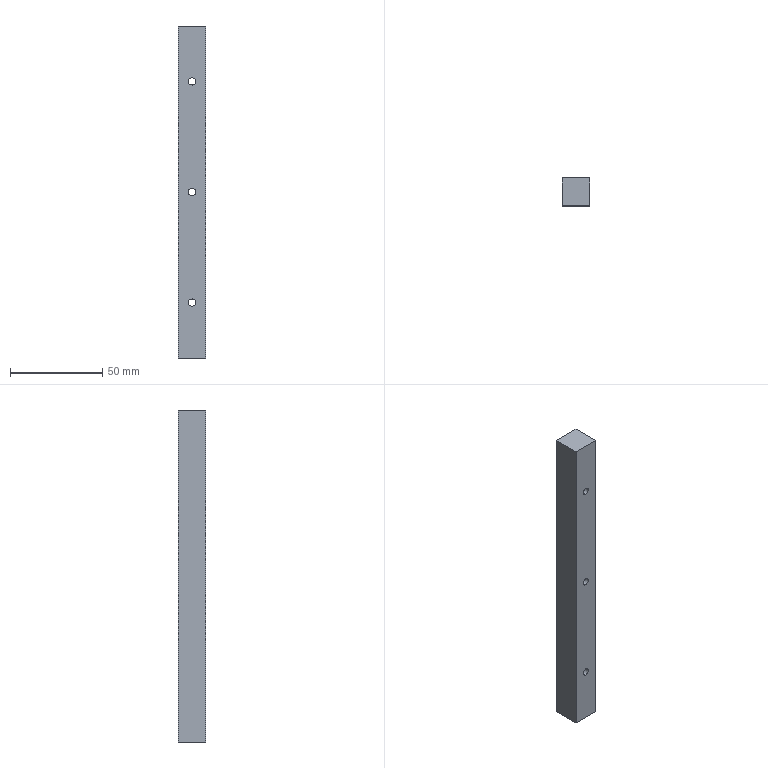Part | SolidWorks | features ICE 2, Extrusion 1, LPattern 1 | 1 solid | 21 faces | box 15 x 15 x 180 mm | volume 39722 mm3 | cylinder 12 | plane 9 | commonest cylinder face diameters 4 x6 6 x6
STEP:
#1=CARTESIAN_POINT('',(0.,-7.5,-62.));
#2=VERTEX_POINT('',#1);
#3=CARTESIAN_POINT('',(0.,-7.5,-58.));
#4=VERTEX_POINT('',#3);
#5=CARTESIAN_POINT('',(0.,-7.5,-60.));
#6=DIRECTION('',(0.,1.,0.));
#7=DIRECTION('',(0.,0.,1.));
#8=AXIS2_PLACEMENT_3D('',#5,#6,#7);
#9=CIRCLE('',#8,2.);
#10=EDGE_CURVE('',#2,#4,#9,.T.);
#11=ORIENTED_EDGE('',*,*,#10,.F.);
#12=CARTESIAN_POINT('',(0.,3.,-62.));
#13=VERTEX_POINT('',#12);
#14=CARTESIAN_POINT('',(0.,-7.5,-62.));
#15=DIRECTION('',(0.,1.,0.));
#16=VECTOR('',#15,1000.);
#17=LINE('',#14,#16);
#18=EDGE_CURVE('',#2,#13,#17,.T.);
#19=ORIENTED_EDGE('',*,*,#18,.T.);
#20=CARTESIAN_POINT('',(0.,3.,-58.));
#21=VERTEX_POINT('',#20);
#22=CARTESIAN_POINT('',(0.,3.,-60.));
#23=DIRECTION('',(0.,1.,0.));
#24=DIRECTION('',(0.,0.,1.));
#25=AXIS2_PLACEMENT_3D('',#22,#23,#24);
#26=CIRCLE('',#25,2.);
#27=EDGE_CURVE('',#13,#21,#26,.T.);
#28=ORIENTED_EDGE('',*,*,#27,.T.);
#29=CARTESIAN_POINT('',(0.,-7.5,-58.));
#30=DIRECTION('',(0.,1.,0.));
#31=VECTOR('',#30,1000.);
#32=LINE('',#29,#31);
#33=EDGE_CURVE('',#4,#21,#32,.T.);
#34=ORIENTED_EDGE('',*,*,#33,.F.);
#35=EDGE_LOOP('',(#11,#19,#28,#34));
#36=FACE_OUTER_BOUND('',#35,.T.);
#37=CARTESIAN_POINT('',(0.,-7.5,-60.));
#38=DIRECTION('',(0.,1.,0.));
#39=DIRECTION('',(0.,0.,1.));
#40=AXIS2_PLACEMENT_3D('',#37,#38,#39);
#41=CYLINDRICAL_SURFACE('',#40,2.);
#42=ADVANCED_FACE('',(#36),#41,.F.);
#43=CARTESIAN_POINT('',(0.,-7.5,-2.));
#44=VERTEX_POINT('',#43);
#45=CARTESIAN_POINT('',(0.,-7.5,2.));
#46=VERTEX_POINT('',#45);
#47=CARTESIAN_POINT('',(0.,-7.5,0.));
#48=DIRECTION('',(0.,1.,0.));
#49=DIRECTION('',(0.,0.,1.));
#50=AXIS2_PLACEMENT_3D('',#47,#48,#49);
#51=CIRCLE('',#50,2.);
#52=EDGE_CURVE('',#44,#46,#51,.T.);
#53=ORIENTED_EDGE('',*,*,#52,.F.);
#54=CARTESIAN_POINT('',(0.,3.,-2.));
#55=VERTEX_POINT('',#54);
#56=CARTESIAN_POINT('',(0.,-7.5,-2.));
#57=DIRECTION('',(0.,1.,0.));
#58=VECTOR('',#57,1000.);
#59=LINE('',#56,#58);
#60=EDGE_CURVE('',#44,#55,#59,.T.);
#61=ORIENTED_EDGE('',*,*,#60,.T.);
#62=CARTESIAN_POINT('',(0.,3.,2.));
#63=VERTEX_POINT('',#62);
#64=CARTESIAN_POINT('',(0.,3.,0.));
#65=DIRECTION('',(0.,1.,0.));
#66=DIRECTION('',(0.,0.,1.));
#67=AXIS2_PLACEMENT_3D('',#64,#65,#66);
#68=CIRCLE('',#67,2.);
#69=EDGE_CURVE('',#55,#63,#68,.T.);
#70=ORIENTED_EDGE('',*,*,#69,.T.);
#71=CARTESIAN_POINT('',(0.,-7.5,2.));
#72=DIRECTION('',(0.,1.,0.));
#73=VECTOR('',#72,1000.);
#74=LINE('',#71,#73);
#75=EDGE_CURVE('',#46,#63,#74,.T.);
#76=ORIENTED_EDGE('',*,*,#75,.F.);
#77=EDGE_LOOP('',(#53,#61,#70,#76));
#78=FACE_OUTER_BOUND('',#77,.T.);
#79=CARTESIAN_POINT('',(0.,-7.5,0.));
#80=DIRECTION('',(0.,1.,0.));
#81=DIRECTION('',(0.,0.,1.));
#82=AXIS2_PLACEMENT_3D('',#79,#80,#81);
#83=CYLINDRICAL_SURFACE('',#82,2.);
#84=ADVANCED_FACE('',(#78),#83,.F.);
#85=CARTESIAN_POINT('',(0.,3.,-63.));
#86=VERTEX_POINT('',#85);
#87=CARTESIAN_POINT('',(0.,3.,-57.));
#88=VERTEX_POINT('',#87);
#89=CARTESIAN_POINT('',(0.,3.,-60.));
#90=DIRECTION('',(0.,1.,0.));
#91=DIRECTION('',(0.,0.,1.));
#92=AXIS2_PLACEMENT_3D('',#89,#90,#91);
#93=CIRCLE('',#92,3.);
#94=EDGE_CURVE('',#86,#88,#93,.T.);
#95=ORIENTED_EDGE('',*,*,#94,.F.);
#96=CARTESIAN_POINT('',(0.,7.5,-63.));
#97=VERTEX_POINT('',#96);
#98=CARTESIAN_POINT('',(0.,3.,-63.));
#99=DIRECTION('',(0.,1.,0.));
#100=VECTOR('',#99,1000.);
#101=LINE('',#98,#100);
#102=EDGE_CURVE('',#86,#97,#101,.T.);
#103=ORIENTED_EDGE('',*,*,#102,.T.);
#104=CARTESIAN_POINT('',(0.,7.5,-57.));
#105=VERTEX_POINT('',#104);
#106=CARTESIAN_POINT('',(0.,7.5,-60.));
#107=DIRECTION('',(0.,1.,0.));
#108=DIRECTION('',(0.,0.,1.));
#109=AXIS2_PLACEMENT_3D('',#106,#107,#108);
#110=CIRCLE('',#109,3.);
#111=EDGE_CURVE('',#97,#105,#110,.T.);
#112=ORIENTED_EDGE('',*,*,#111,.T.);
#113=CARTESIAN_POINT('',(0.,3.,-57.));
#114=DIRECTION('',(0.,1.,0.));
#115=VECTOR('',#114,1000.);
#116=LINE('',#113,#115);
#117=EDGE_CURVE('',#88,#105,#116,.T.);
#118=ORIENTED_EDGE('',*,*,#117,.F.);
#119=EDGE_LOOP('',(#95,#103,#112,#118));
#120=FACE_OUTER_BOUND('',#119,.T.);
#121=CARTESIAN_POINT('',(0.,3.,-60.));
#122=DIRECTION('',(0.,1.,0.));
#123=DIRECTION('',(0.,0.,1.));
#124=AXIS2_PLACEMENT_3D('',#121,#122,#123);
#125=CYLINDRICAL_SURFACE('',#124,3.);
#126=ADVANCED_FACE('',(#120),#125,.F.);
#127=CARTESIAN_POINT('',(0.,3.,-3.));
#128=VERTEX_POINT('',#127);
#129=CARTESIAN_POINT('',(0.,3.,3.));
#130=VERTEX_POINT('',#129);
#131=CARTESIAN_POINT('',(0.,3.,0.));
#132=DIRECTION('',(0.,1.,0.));
#133=DIRECTION('',(0.,0.,1.));
#134=AXIS2_PLACEMENT_3D('',#131,#132,#133);
#135=CIRCLE('',#134,3.);
#136=EDGE_CURVE('',#128,#130,#135,.T.);
#137=ORIENTED_EDGE('',*,*,#136,.F.);
#138=CARTESIAN_POINT('',(0.,7.5,-3.));
#139=VERTEX_POINT('',#138);
#140=CARTESIAN_POINT('',(0.,3.,-3.));
#141=DIRECTION('',(0.,1.,0.));
#142=VECTOR('',#141,1000.);
#143=LINE('',#140,#142);
#144=EDGE_CURVE('',#128,#139,#143,.T.);
#145=ORIENTED_EDGE('',*,*,#144,.T.);
#146=CARTESIAN_POINT('',(0.,7.5,3.));
#147=VERTEX_POINT('',#146);
#148=CARTESIAN_POINT('',(0.,7.5,0.));
#149=DIRECTION('',(0.,1.,0.));
#150=DIRECTION('',(0.,0.,1.));
#151=AXIS2_PLACEMENT_3D('',#148,#149,#150);
#152=CIRCLE('',#151,3.);
#153=EDGE_CURVE('',#139,#147,#152,.T.);
#154=ORIENTED_EDGE('',*,*,#153,.T.);
#155=CARTESIAN_POINT('',(0.,3.,3.));
#156=DIRECTION('',(0.,1.,0.));
#157=VECTOR('',#156,1000.);
#158=LINE('',#155,#157);
#159=EDGE_CURVE('',#130,#147,#158,.T.);
#160=ORIENTED_EDGE('',*,*,#159,.F.);
#161=EDGE_LOOP('',(#137,#145,#154,#160));
#162=FACE_OUTER_BOUND('',#161,.T.);
#163=CARTESIAN_POINT('',(0.,3.,0.));
#164=DIRECTION('',(0.,1.,0.));
#165=DIRECTION('',(0.,0.,1.));
#166=AXIS2_PLACEMENT_3D('',#163,#164,#165);
#167=CYLINDRICAL_SURFACE('',#166,3.);
#168=ADVANCED_FACE('',(#162),#167,.F.);
#169=CARTESIAN_POINT('',(0.,-7.5,58.));
#170=VERTEX_POINT('',#169);
#171=CARTESIAN_POINT('',(0.,-7.5,62.));
#172=VERTEX_POINT('',#171);
#173=CARTESIAN_POINT('',(0.,-7.5,60.));
#174=DIRECTION('',(0.,1.,0.));
#175=DIRECTION('',(0.,0.,1.));
#176=AXIS2_PLACEMENT_3D('',#173,#174,#175);
#177=CIRCLE('',#176,2.);
#178=EDGE_CURVE('',#170,#172,#177,.T.);
#179=ORIENTED_EDGE('',*,*,#178,.F.);
#180=CARTESIAN_POINT('',(0.,3.,58.));
#181=VERTEX_POINT('',#180);
#182=CARTESIAN_POINT('',(0.,-7.5,58.));
#183=DIRECTION('',(0.,1.,0.));
#184=VECTOR('',#183,1000.);
#185=LINE('',#182,#184);
#186=EDGE_CURVE('',#170,#181,#185,.T.);
#187=ORIENTED_EDGE('',*,*,#186,.T.);
#188=CARTESIAN_POINT('',(0.,3.,62.));
#189=VERTEX_POINT('',#188);
#190=CARTESIAN_POINT('',(0.,3.,60.));
#191=DIRECTION('',(0.,1.,0.));
#192=DIRECTION('',(0.,0.,1.));
#193=AXIS2_PLACEMENT_3D('',#190,#191,#192);
#194=CIRCLE('',#193,2.);
#195=EDGE_CURVE('',#181,#189,#194,.T.);
#196=ORIENTED_EDGE('',*,*,#195,.T.);
#197=CARTESIAN_POINT('',(0.,-7.5,62.));
#198=DIRECTION('',(0.,1.,0.));
#199=VECTOR('',#198,1000.);
#200=LINE('',#197,#199);
#201=EDGE_CURVE('',#172,#189,#200,.T.);
#202=ORIENTED_EDGE('',*,*,#201,.F.);
#203=EDGE_LOOP('',(#179,#187,#196,#202));
#204=FACE_OUTER_BOUND('',#203,.T.);
#205=CARTESIAN_POINT('',(0.,-7.5,60.));
#206=DIRECTION('',(0.,1.,0.));
#207=DIRECTION('',(0.,0.,1.));
#208=AXIS2_PLACEMENT_3D('',#205,#206,#207);
#209=CYLINDRICAL_SURFACE('',#208,2.);
#210=ADVANCED_FACE('',(#204),#209,.F.);
#211=CARTESIAN_POINT('',(0.,3.,57.));
#212=VERTEX_POINT('',#211);
#213=CARTESIAN_POINT('',(0.,3.,63.));
#214=VERTEX_POINT('',#213);
#215=CARTESIAN_POINT('',(0.,3.,60.));
#216=DIRECTION('',(0.,1.,0.));
#217=DIRECTION('',(0.,0.,1.));
#218=AXIS2_PLACEMENT_3D('',#215,#216,#217);
#219=CIRCLE('',#218,3.);
#220=EDGE_CURVE('',#212,#214,#219,.T.);
#221=ORIENTED_EDGE('',*,*,#220,.F.);
#222=CARTESIAN_POINT('',(0.,7.5,57.));
#223=VERTEX_POINT('',#222);
#224=CARTESIAN_POINT('',(0.,3.,57.));
#225=DIRECTION('',(0.,1.,0.));
#226=VECTOR('',#225,1000.);
#227=LINE('',#224,#226);
#228=EDGE_CURVE('',#212,#223,#227,.T.);
#229=ORIENTED_EDGE('',*,*,#228,.T.);
#230=CARTESIAN_POINT('',(0.,7.5,63.));
#231=VERTEX_POINT('',#230);
#232=CARTESIAN_POINT('',(0.,7.5,60.));
#233=DIRECTION('',(0.,1.,0.));
#234=DIRECTION('',(0.,0.,1.));
#235=AXIS2_PLACEMENT_3D('',#232,#233,#234);
#236=CIRCLE('',#235,3.);
#237=EDGE_CURVE('',#223,#231,#236,.T.);
#238=ORIENTED_EDGE('',*,*,#237,.T.);
#239=CARTESIAN_POINT('',(0.,3.,63.));
#240=DIRECTION('',(0.,1.,0.));
#241=VECTOR('',#240,1000.);
#242=LINE('',#239,#241);
#243=EDGE_CURVE('',#214,#231,#242,.T.);
#244=ORIENTED_EDGE('',*,*,#243,.F.);
#245=EDGE_LOOP('',(#221,#229,#238,#244));
#246=FACE_OUTER_BOUND('',#245,.T.);
#247=CARTESIAN_POINT('',(0.,3.,60.));
#248=DIRECTION('',(0.,1.,0.));
#249=DIRECTION('',(0.,0.,1.));
#250=AXIS2_PLACEMENT_3D('',#247,#248,#249);
#251=CYLINDRICAL_SURFACE('',#250,3.);
#252=ADVANCED_FACE('',(#246),#251,.F.);
#253=CARTESIAN_POINT('',(7.5,-7.5,-90.));
#254=VERTEX_POINT('',#253);
#255=CARTESIAN_POINT('',(7.5,7.5,-90.));
#256=VERTEX_POINT('',#255);
#257=CARTESIAN_POINT('',(7.5,7.5,-90.));
#258=DIRECTION('',(0.,1.,0.));
#259=VECTOR('',#258,1000.);
#260=LINE('',#257,#259);
#261=EDGE_CURVE('',#254,#256,#260,.T.);
#262=ORIENTED_EDGE('',*,*,#261,.T.);
#263=CARTESIAN_POINT('',(7.5,7.5,90.));
#264=VERTEX_POINT('',#263);
#265=CARTESIAN_POINT('',(7.5,7.5,90.));
#266=DIRECTION('',(0.,0.,-1.));
#267=VECTOR('',#266,1000.);
#268=LINE('',#265,#267);
#269=EDGE_CURVE('',#264,#256,#268,.T.);
#270=ORIENTED_EDGE('',*,*,#269,.F.);
#271=CARTESIAN_POINT('',(7.5,-7.5,90.));
#272=VERTEX_POINT('',#271);
#273=CARTESIAN_POINT('',(7.5,7.5,90.));
#274=DIRECTION('',(0.,1.,0.));
#275=VECTOR('',#274,1000.);
#276=LINE('',#273,#275);
#277=EDGE_CURVE('',#272,#264,#276,.T.);
#278=ORIENTED_EDGE('',*,*,#277,.F.);
#279=CARTESIAN_POINT('',(7.5,-7.5,90.));
#280=DIRECTION('',(0.,0.,-1.));
#281=VECTOR('',#280,1000.);
#282=LINE('',#279,#281);
#283=EDGE_CURVE('',#272,#254,#282,.T.);
#284=ORIENTED_EDGE('',*,*,#283,.T.);
#285=EDGE_LOOP('',(#262,#270,#278,#284));
#286=FACE_OUTER_BOUND('',#285,.T.);
#287=CARTESIAN_POINT('',(7.5,7.5,90.));
#288=DIRECTION('',(-1.,0.,0.));
#289=DIRECTION('',(0.,-1.,0.));
#290=AXIS2_PLACEMENT_3D('',#287,#288,#289);
#291=PLANE('',#290);
#292=ADVANCED_FACE('',(#286),#291,.F.);
#293=CARTESIAN_POINT('',(0.,7.5,-60.));
#294=DIRECTION('',(0.,1.,0.));
#295=DIRECTION('',(0.,0.,1.));
#296=AXIS2_PLACEMENT_3D('',#293,#294,#295);
#297=CIRCLE('',#296,3.);
#298=EDGE_CURVE('',#105,#97,#297,.T.);
#299=ORIENTED_EDGE('',*,*,#298,.F.);
#300=ORIENTED_EDGE('',*,*,#111,.F.);
#301=EDGE_LOOP('',(#299,#300));
#302=FACE_BOUND('',#301,.T.);
#303=CARTESIAN_POINT('',(0.,7.5,0.));
#304=DIRECTION('',(0.,1.,0.));
#305=DIRECTION('',(0.,0.,1.));
#306=AXIS2_PLACEMENT_3D('',#303,#304,#305);
#307=CIRCLE('',#306,3.);
#308=EDGE_CURVE('',#147,#139,#307,.T.);
#309=ORIENTED_EDGE('',*,*,#308,.F.);
#310=ORIENTED_EDGE('',*,*,#153,.F.);
#311=EDGE_LOOP('',(#309,#310));
#312=FACE_BOUND('',#311,.T.);
#313=CARTESIAN_POINT('',(0.,7.5,60.));
#314=DIRECTION('',(0.,1.,0.));
#315=DIRECTION('',(0.,0.,1.));
#316=AXIS2_PLACEMENT_3D('',#313,#314,#315);
#317=CIRCLE('',#316,3.);
#318=EDGE_CURVE('',#231,#223,#317,.T.);
#319=ORIENTED_EDGE('',*,*,#318,.F.);
#320=ORIENTED_EDGE('',*,*,#237,.F.);
#321=EDGE_LOOP('',(#319,#320));
#322=FACE_BOUND('',#321,.T.);
#323=CARTESIAN_POINT('',(-7.5,7.5,-90.));
#324=VERTEX_POINT('',#323);
#325=CARTESIAN_POINT('',(-7.5,7.5,-90.));
#326=DIRECTION('',(-1.,0.,0.));
#327=VECTOR('',#326,1000.);
#328=LINE('',#325,#327);
#329=EDGE_CURVE('',#256,#324,#328,.T.);
#330=ORIENTED_EDGE('',*,*,#329,.T.);
#331=CARTESIAN_POINT('',(-7.5,7.5,90.));
#332=VERTEX_POINT('',#331);
#333=CARTESIAN_POINT('',(-7.5,7.5,90.));
#334=DIRECTION('',(0.,0.,-1.));
#335=VECTOR('',#334,1000.);
#336=LINE('',#333,#335);
#337=EDGE_CURVE('',#332,#324,#336,.T.);
#338=ORIENTED_EDGE('',*,*,#337,.F.);
#339=CARTESIAN_POINT('',(-7.5,7.5,90.));
#340=DIRECTION('',(-1.,0.,0.));
#341=VECTOR('',#340,1000.);
#342=LINE('',#339,#341);
#343=EDGE_CURVE('',#264,#332,#342,.T.);
#344=ORIENTED_EDGE('',*,*,#343,.F.);
#345=ORIENTED_EDGE('',*,*,#269,.T.);
#346=EDGE_LOOP('',(#330,#338,#344,#345));
#347=FACE_OUTER_BOUND('',#346,.T.);
#348=CARTESIAN_POINT('',(-7.5,7.5,90.));
#349=DIRECTION('',(0.,-1.,0.));
#350=DIRECTION('',(0.,0.,-1.));
#351=AXIS2_PLACEMENT_3D('',#348,#349,#350);
#352=PLANE('',#351);
#353=ADVANCED_FACE('',(#302,#312,#322,#347),#352,.F.);
#354=CARTESIAN_POINT('',(-7.5,-7.5,-90.));
#355=VERTEX_POINT('',#354);
#356=CARTESIAN_POINT('',(-7.5,7.5,-90.));
#357=DIRECTION('',(0.,-1.,0.));
#358=VECTOR('',#357,1000.);
#359=LINE('',#356,#358);
#360=EDGE_CURVE('',#324,#355,#359,.T.);
#361=ORIENTED_EDGE('',*,*,#360,.T.);
#362=CARTESIAN_POINT('',(-7.5,-7.5,90.));
#363=VERTEX_POINT('',#362);
#364=CARTESIAN_POINT('',(-7.5,-7.5,90.));
#365=DIRECTION('',(0.,0.,-1.));
#366=VECTOR('',#365,1000.);
#367=LINE('',#364,#366);
#368=EDGE_CURVE('',#363,#355,#367,.T.);
#369=ORIENTED_EDGE('',*,*,#368,.F.);
#370=CARTESIAN_POINT('',(-7.5,7.5,90.));
#371=DIRECTION('',(0.,-1.,0.));
#372=VECTOR('',#371,1000.);
#373=LINE('',#370,#372);
#374=EDGE_CURVE('',#332,#363,#373,.T.);
#375=ORIENTED_EDGE('',*,*,#374,.F.);
#376=ORIENTED_EDGE('',*,*,#337,.T.);
#377=EDGE_LOOP('',(#361,#369,#375,#376));
#378=FACE_OUTER_BOUND('',#377,.T.);
#379=CARTESIAN_POINT('',(-7.5,7.5,90.));
#380=DIRECTION('',(1.,0.,0.));
#381=DIRECTION('',(0.,1.,0.));
#382=AXIS2_PLACEMENT_3D('',#379,#380,#381);
#383=PLANE('',#382);
#384=ADVANCED_FACE('',(#378),#383,.F.);
#385=CARTESIAN_POINT('',(0.,-7.5,-60.));
#386=DIRECTION('',(0.,1.,0.));
#387=DIRECTION('',(0.,0.,1.));
#388=AXIS2_PLACEMENT_3D('',#385,#386,#387);
#389=CIRCLE('',#388,2.);
#390=EDGE_CURVE('',#4,#2,#389,.T.);
#391=ORIENTED_EDGE('',*,*,#390,.T.);
#392=ORIENTED_EDGE('',*,*,#10,.T.);
#393=EDGE_LOOP('',(#391,#392));
#394=FACE_BOUND('',#393,.T.);
#395=CARTESIAN_POINT('',(0.,-7.5,0.));
#396=DIRECTION('',(0.,1.,0.));
#397=DIRECTION('',(0.,0.,1.));
#398=AXIS2_PLACEMENT_3D('',#395,#396,#397);
#399=CIRCLE('',#398,2.);
#400=EDGE_CURVE('',#46,#44,#399,.T.);
#401=ORIENTED_EDGE('',*,*,#400,.T.);
#402=ORIENTED_EDGE('',*,*,#52,.T.);
#403=EDGE_LOOP('',(#401,#402));
#404=FACE_BOUND('',#403,.T.);
#405=CARTESIAN_POINT('',(0.,-7.5,60.));
#406=DIRECTION('',(0.,1.,0.));
#407=DIRECTION('',(0.,0.,1.));
#408=AXIS2_PLACEMENT_3D('',#405,#406,#407);
#409=CIRCLE('',#408,2.);
#410=EDGE_CURVE('',#172,#170,#409,.T.);
#411=ORIENTED_EDGE('',*,*,#410,.T.);
#412=ORIENTED_EDGE('',*,*,#178,.T.);
#413=EDGE_LOOP('',(#411,#412));
#414=FACE_BOUND('',#413,.T.);
#415=CARTESIAN_POINT('',(-7.5,-7.5,-90.));
#416=DIRECTION('',(1.,0.,0.));
#417=VECTOR('',#416,1000.);
#418=LINE('',#415,#417);
#419=EDGE_CURVE('',#355,#254,#418,.T.);
#420=ORIENTED_EDGE('',*,*,#419,.T.);
#421=ORIENTED_EDGE('',*,*,#283,.F.);
#422=CARTESIAN_POINT('',(-7.5,-7.5,90.));
#423=DIRECTION('',(1.,0.,0.));
#424=VECTOR('',#423,1000.);
#425=LINE('',#422,#424);
#426=EDGE_CURVE('',#363,#272,#425,.T.);
#427=ORIENTED_EDGE('',*,*,#426,.F.);
#428=ORIENTED_EDGE('',*,*,#368,.T.);
#429=EDGE_LOOP('',(#420,#421,#427,#428));
#430=FACE_OUTER_BOUND('',#429,.T.);
#431=CARTESIAN_POINT('',(-7.5,-7.5,90.));
#432=DIRECTION('',(0.,1.,0.));
#433=DIRECTION('',(0.,0.,1.));
#434=AXIS2_PLACEMENT_3D('',#431,#432,#433);
#435=PLANE('',#434);
#436=ADVANCED_FACE('',(#394,#404,#414,#430),#435,.F.);
#437=ORIENTED_EDGE('',*,*,#277,.T.);
#438=ORIENTED_EDGE('',*,*,#343,.T.);
#439=ORIENTED_EDGE('',*,*,#374,.T.);
#440=ORIENTED_EDGE('',*,*,#426,.T.);
#441=EDGE_LOOP('',(#437,#438,#439,#440));
#442=FACE_OUTER_BOUND('',#441,.T.);
#443=CARTESIAN_POINT('',(0.,0.,90.));
#444=DIRECTION('',(0.,0.,1.));
#445=DIRECTION('',(1.,0.,0.));
#446=AXIS2_PLACEMENT_3D('',#443,#444,#445);
#447=PLANE('',#446);
#448=ADVANCED_FACE('',(#442),#447,.T.);
#449=ORIENTED_EDGE('',*,*,#261,.F.);
#450=ORIENTED_EDGE('',*,*,#419,.F.);
#451=ORIENTED_EDGE('',*,*,#360,.F.);
#452=ORIENTED_EDGE('',*,*,#329,.F.);
#453=EDGE_LOOP('',(#449,#450,#451,#452));
#454=FACE_OUTER_BOUND('',#453,.T.);
#455=CARTESIAN_POINT('',(0.,0.,-90.));
#456=DIRECTION('',(0.,0.,1.));
#457=DIRECTION('',(1.,0.,0.));
#458=AXIS2_PLACEMENT_3D('',#455,#456,#457);
#459=PLANE('',#458);
#460=ADVANCED_FACE('',(#454),#459,.F.);
#461=ORIENTED_EDGE('',*,*,#228,.F.);
#462=CARTESIAN_POINT('',(0.,3.,60.));
#463=DIRECTION('',(0.,1.,0.));
#464=DIRECTION('',(0.,0.,1.));
#465=AXIS2_PLACEMENT_3D('',#462,#463,#464);
#466=CIRCLE('',#465,3.);
#467=EDGE_CURVE('',#214,#212,#466,.T.);
#468=ORIENTED_EDGE('',*,*,#467,.F.);
#469=ORIENTED_EDGE('',*,*,#243,.T.);
#470=ORIENTED_EDGE('',*,*,#318,.T.);
#471=EDGE_LOOP('',(#461,#468,#469,#470));
#472=FACE_OUTER_BOUND('',#471,.T.);
#473=CARTESIAN_POINT('',(0.,3.,60.));
#474=DIRECTION('',(0.,1.,0.));
#475=DIRECTION('',(0.,0.,1.));
#476=AXIS2_PLACEMENT_3D('',#473,#474,#475);
#477=CYLINDRICAL_SURFACE('',#476,3.);
#478=ADVANCED_FACE('',(#472),#477,.F.);
#479=CARTESIAN_POINT('',(0.,3.,60.));
#480=DIRECTION('',(0.,1.,0.));
#481=DIRECTION('',(0.,0.,1.));
#482=AXIS2_PLACEMENT_3D('',#479,#480,#481);
#483=CIRCLE('',#482,2.);
#484=EDGE_CURVE('',#189,#181,#483,.T.);
#485=ORIENTED_EDGE('',*,*,#484,.F.);
#486=ORIENTED_EDGE('',*,*,#195,.F.);
#487=EDGE_LOOP('',(#485,#486));
#488=FACE_BOUND('',#487,.T.);
#489=ORIENTED_EDGE('',*,*,#467,.T.);
#490=ORIENTED_EDGE('',*,*,#220,.T.);
#491=EDGE_LOOP('',(#489,#490));
#492=FACE_OUTER_BOUND('',#491,.T.);
#493=CARTESIAN_POINT('',(0.,3.,60.));
#494=DIRECTION('',(0.,1.,0.));
#495=DIRECTION('',(0.,0.,1.));
#496=AXIS2_PLACEMENT_3D('',#493,#494,#495);
#497=PLANE('',#496);
#498=ADVANCED_FACE('',(#488,#492),#497,.T.);
#499=ORIENTED_EDGE('',*,*,#186,.F.);
#500=ORIENTED_EDGE('',*,*,#410,.F.);
#501=ORIENTED_EDGE('',*,*,#201,.T.);
#502=ORIENTED_EDGE('',*,*,#484,.T.);
#503=EDGE_LOOP('',(#499,#500,#501,#502));
#504=FACE_OUTER_BOUND('',#503,.T.);
#505=CARTESIAN_POINT('',(0.,-7.5,60.));
#506=DIRECTION('',(0.,1.,0.));
#507=DIRECTION('',(0.,0.,1.));
#508=AXIS2_PLACEMENT_3D('',#505,#506,#507);
#509=CYLINDRICAL_SURFACE('',#508,2.);
#510=ADVANCED_FACE('',(#504),#509,.F.);
#511=ORIENTED_EDGE('',*,*,#144,.F.);
#512=CARTESIAN_POINT('',(0.,3.,0.));
#513=DIRECTION('',(0.,1.,0.));
#514=DIRECTION('',(0.,0.,1.));
#515=AXIS2_PLACEMENT_3D('',#512,#513,#514);
#516=CIRCLE('',#515,3.);
#517=EDGE_CURVE('',#130,#128,#516,.T.);
#518=ORIENTED_EDGE('',*,*,#517,.F.);
#519=ORIENTED_EDGE('',*,*,#159,.T.);
#520=ORIENTED_EDGE('',*,*,#308,.T.);
#521=EDGE_LOOP('',(#511,#518,#519,#520));
#522=FACE_OUTER_BOUND('',#521,.T.);
#523=CARTESIAN_POINT('',(0.,3.,0.));
#524=DIRECTION('',(0.,1.,0.));
#525=DIRECTION('',(0.,0.,1.));
#526=AXIS2_PLACEMENT_3D('',#523,#524,#525);
#527=CYLINDRICAL_SURFACE('',#526,3.);
#528=ADVANCED_FACE('',(#522),#527,.F.);
#529=CARTESIAN_POINT('',(0.,3.,0.));
#530=DIRECTION('',(0.,1.,0.));
#531=DIRECTION('',(0.,0.,1.));
#532=AXIS2_PLACEMENT_3D('',#529,#530,#531);
#533=CIRCLE('',#532,2.);
#534=EDGE_CURVE('',#63,#55,#533,.T.);
#535=ORIENTED_EDGE('',*,*,#534,.F.);
#536=ORIENTED_EDGE('',*,*,#69,.F.);
#537=EDGE_LOOP('',(#535,#536));
#538=FACE_BOUND('',#537,.T.);
#539=ORIENTED_EDGE('',*,*,#517,.T.);
#540=ORIENTED_EDGE('',*,*,#136,.T.);
#541=EDGE_LOOP('',(#539,#540));
#542=FACE_OUTER_BOUND('',#541,.T.);
#543=CARTESIAN_POINT('',(0.,3.,0.));
#544=DIRECTION('',(0.,1.,0.));
#545=DIRECTION('',(0.,0.,1.));
#546=AXIS2_PLACEMENT_3D('',#543,#544,#545);
#547=PLANE('',#546);
#548=ADVANCED_FACE('',(#538,#542),#547,.T.);
#549=ORIENTED_EDGE('',*,*,#102,.F.);
#550=CARTESIAN_POINT('',(0.,3.,-60.));
#551=DIRECTION('',(0.,1.,0.));
#552=DIRECTION('',(0.,0.,1.));
#553=AXIS2_PLACEMENT_3D('',#550,#551,#552);
#554=CIRCLE('',#553,3.);
#555=EDGE_CURVE('',#88,#86,#554,.T.);
#556=ORIENTED_EDGE('',*,*,#555,.F.);
#557=ORIENTED_EDGE('',*,*,#117,.T.);
#558=ORIENTED_EDGE('',*,*,#298,.T.);
#559=EDGE_LOOP('',(#549,#556,#557,#558));
#560=FACE_OUTER_BOUND('',#559,.T.);
#561=CARTESIAN_POINT('',(0.,3.,-60.));
#562=DIRECTION('',(0.,1.,0.));
#563=DIRECTION('',(0.,0.,1.));
#564=AXIS2_PLACEMENT_3D('',#561,#562,#563);
#565=CYLINDRICAL_SURFACE('',#564,3.);
#566=ADVANCED_FACE('',(#560),#565,.F.);
#567=CARTESIAN_POINT('',(0.,3.,-60.));
#568=DIRECTION('',(0.,1.,0.));
#569=DIRECTION('',(0.,0.,1.));
#570=AXIS2_PLACEMENT_3D('',#567,#568,#569);
#571=CIRCLE('',#570,2.);
#572=EDGE_CURVE('',#21,#13,#571,.T.);
#573=ORIENTED_EDGE('',*,*,#572,.F.);
#574=ORIENTED_EDGE('',*,*,#27,.F.);
#575=EDGE_LOOP('',(#573,#574));
#576=FACE_BOUND('',#575,.T.);
#577=ORIENTED_EDGE('',*,*,#555,.T.);
#578=ORIENTED_EDGE('',*,*,#94,.T.);
#579=EDGE_LOOP('',(#577,#578));
#580=FACE_OUTER_BOUND('',#579,.T.);
#581=CARTESIAN_POINT('',(0.,3.,-60.));
#582=DIRECTION('',(0.,1.,0.));
#583=DIRECTION('',(0.,0.,1.));
#584=AXIS2_PLACEMENT_3D('',#581,#582,#583);
#585=PLANE('',#584);
#586=ADVANCED_FACE('',(#576,#580),#585,.T.);
#587=ORIENTED_EDGE('',*,*,#60,.F.);
#588=ORIENTED_EDGE('',*,*,#400,.F.);
#589=ORIENTED_EDGE('',*,*,#75,.T.);
#590=ORIENTED_EDGE('',*,*,#534,.T.);
#591=EDGE_LOOP('',(#587,#588,#589,#590));
#592=FACE_OUTER_BOUND('',#591,.T.);
#593=CARTESIAN_POINT('',(0.,-7.5,0.));
#594=DIRECTION('',(0.,1.,0.));
#595=DIRECTION('',(0.,0.,1.));
#596=AXIS2_PLACEMENT_3D('',#593,#594,#595);
#597=CYLINDRICAL_SURFACE('',#596,2.);
#598=ADVANCED_FACE('',(#592),#597,.F.);
#599=ORIENTED_EDGE('',*,*,#18,.F.);
#600=ORIENTED_EDGE('',*,*,#390,.F.);
#601=ORIENTED_EDGE('',*,*,#33,.T.);
#602=ORIENTED_EDGE('',*,*,#572,.T.);
#603=EDGE_LOOP('',(#599,#600,#601,#602));
#604=FACE_OUTER_BOUND('',#603,.T.);
#605=CARTESIAN_POINT('',(0.,-7.5,-60.));
#606=DIRECTION('',(0.,1.,0.));
#607=DIRECTION('',(0.,0.,1.));
#608=AXIS2_PLACEMENT_3D('',#605,#606,#607);
#609=CYLINDRICAL_SURFACE('',#608,2.);
#610=ADVANCED_FACE('',(#604),#609,.F.);
#611=CLOSED_SHELL('',(#42,#84,#126,#168,#210,#252,#292,#353,#384,#436,#448,#460,#478,#498,#510,#528,#548,#566,#586,#598,#610));
#612=MANIFOLD_SOLID_BREP('',#611);
#613=CARTESIAN_POINT('',(0.,0.,0.));
#614=DIRECTION('',(0.,0.,1.));
#615=DIRECTION('',(1.,0.,0.));
#616=AXIS2_PLACEMENT_3D('',#613,#614,#615);
#617=(LENGTH_UNIT()NAMED_UNIT(*)SI_UNIT(.MILLI.,.METRE.));
#618=UNCERTAINTY_MEASURE_WITH_UNIT(LENGTH_MEASURE(0.00001),#617,'','');
#619=(NAMED_UNIT(*)PLANE_ANGLE_UNIT()SI_UNIT($,.RADIAN.));
#620=(NAMED_UNIT(*)SI_UNIT($,.STERADIAN.)SOLID_ANGLE_UNIT());
#621=(GEOMETRIC_REPRESENTATION_CONTEXT(3)GLOBAL_UNCERTAINTY_ASSIGNED_CONTEXT((#618))GLOBAL_UNIT_ASSIGNED_CONTEXT((#617,#619,#620))REPRESENTATION_CONTEXT('',''));
#622=ADVANCED_BREP_SHAPE_REPRESENTATION('',(#612,#616),#621);